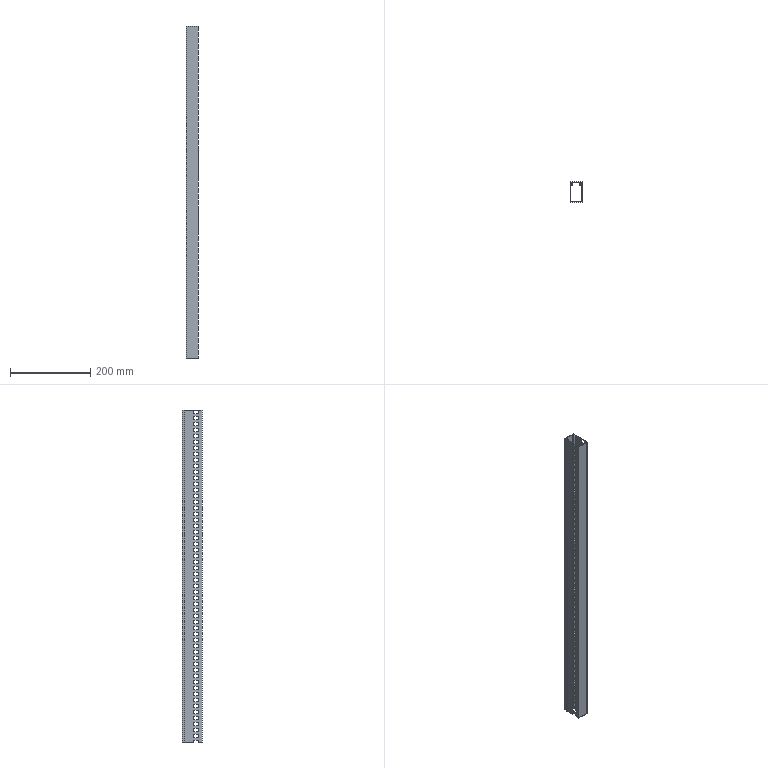Part | SolidWorks | features BaseBody 1 | 1 solid | 473 faces | box 30 x 50 x 830 mm | volume 135173 mm3 | plane 249 | cylinder 224 | commonest cylinder face diameters 8 x224